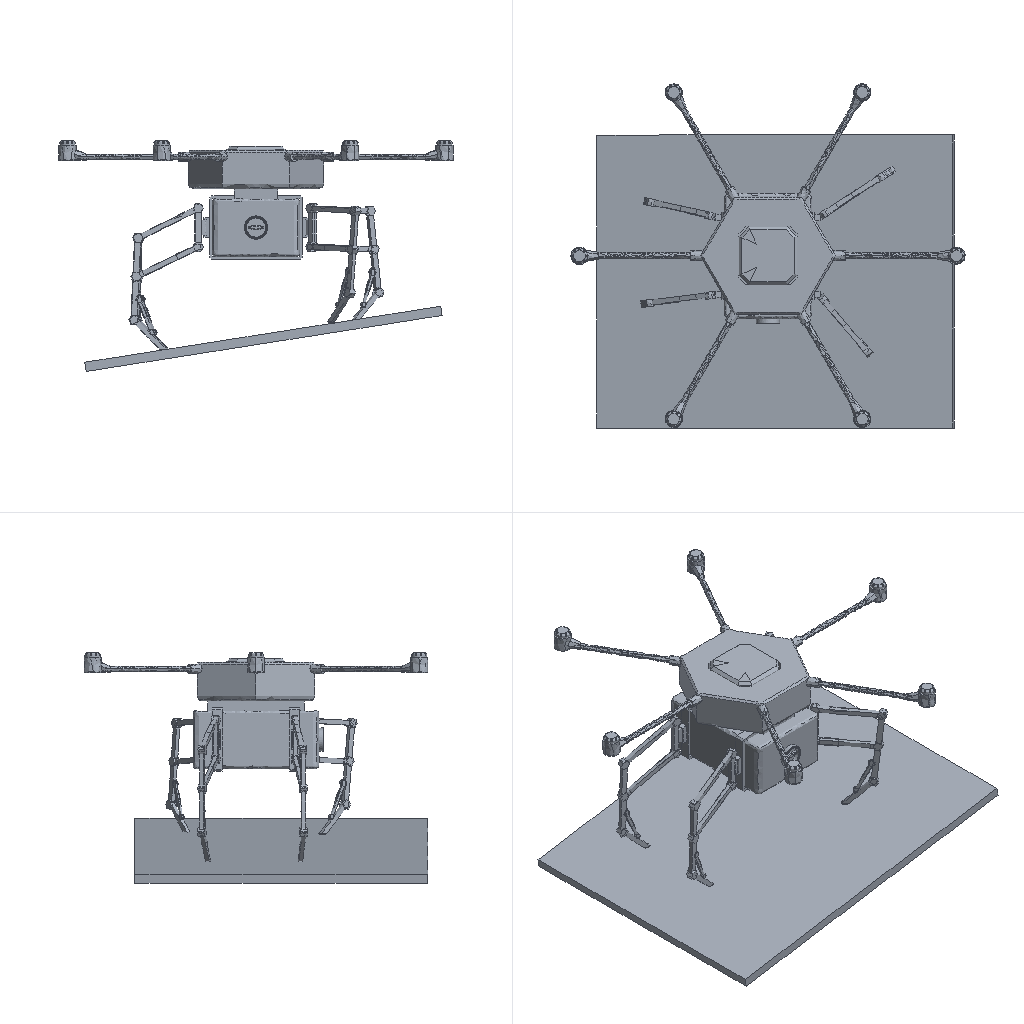Simulation study | ansys workbench
Ansys APDL input file, long lists of numbers shortened:
/batch
/config,noeldb,1     ! force off writing results to database
*get,_wallstrt,active,,time,wall
! ANSYS input file written by Workbench version 2022 R1
! File used for geometry attach:
/title,wbnew--____ (B5)
! ****** Begin Custom Load Command Snippet ******
/COM, ACT Extensions:
/COM,     LSDYNA, 2021.1
/COM,
! ****** End   Custom Load Command Snippet ******
*DIM,_wb_ProjectScratch_dir,string,248
_wb_ProjectScratch_dir(1) = ''
*DIM,_wb_SolverFiles_dir,string,248
_wb_SolverFiles_dir(1) = ''
*DIM,_wb_userfiles_dir,string,248
_wb_userfiles_dir(1) = ''
/com,--- Data in consistent NMM units. See Solving Units in the help system for more information.
/units,MPA
/nopr
/wb,file,start              !  signify a WB generated input file
/prep7
! Turn off shape checking because checks already performed inside WB mesher.
! See help system for more information.
SHPP,OFF,,NOWARN
/nolist
etcon,set             ! allow ANSYS to choose best KEYOP's for 180x elements, resets any applicable keyopt to MAPDL defaults
/com,*********** Nodes for the whole assembly ***********
nblock,3,,112162
(1i9,3e20.9e3)
        1    -4.940198886E+03     5.343852573E+02    -1.661004366E+03
! (101965 more lines like these left out)
-1
/wb,elem,start            !  set before creation of elements
/com,*********** Elements for Body 1 "xuanyi|dianjizhijia|Chamfer.1" ***********
et,1,187
eblock,19,solid,,480
(19i9)
        1        1        1        1        0        0        0        0       10        0    20386    35761    35765    35869    35796    35956    35983    35959    35957
! (959 more lines like these left out)
-1
/com,*********** Elements for Body 2 "xuanyi|jibi|Pad.1" ***********
et,2,187
eblock,19,solid,,1308
(19i9)
        2        2        2        2        0        0        0        0       10        0    42182    78115    78116    78183    78275    79189    79200    79191    79195
! (2615 more lines like these left out)
-1
/com,*********** Elements for Body 3 "xuanyi|xuanyidianji|CircPattern.1" ***********
et,3,187
eblock,19,solid,,3493
(19i9)
        3        3        3        3        0        0        0        0       10        0     9130    17713    17730    17812    17778    22405    22473    22409    22406
! (6985 more lines like these left out)
-1
/com,*********** Elements for Body 4 "xuanyi|dianjizhijia|Chamfer.1[2]" ***********
et,4,187
eblock,19,solid,,480
(19i9)
        4        4        4        4        0        0        0        0       10        0     4107     6963     6967     7071     6998     7158     7185     7161     7159
! (959 more lines like these left out)
-1
/com,*********** Elements for Body 5 "xuanyi|jibi|Pad.1[2]" ***********
et,5,187
eblock,19,solid,,1308
(19i9)
        5        5        5        5        0        0        0        0       10        0    40874    75480    75481    75548    75640    76554    76565    76556    76560
! (2615 more lines like these left out)
-1
! (50 more sections like these left out)
/wb,elem,end               !  done creating elements
/com,*********** Send User Defined Coordinate System(s) ***********
csys,0
toffst,273.15,  ! Temperature offset from absolute zero
/com,*********** Set Reference Temperature ***********
tref,22.
/wb,mat,start              !  starting to send materials
/com,*********** Send Materials ***********
Temperature = 'TEMP' ! Temperature
MP,DENS,1,7.85e-09,	! tonne mm^-3
MP,ALPX,1,1.2e-05,	! C^-1
MP,C,1,434000000,	! mm^2 s^-2 C^-1
MP,KXX,1,60.5,	! tonne mm s^-3 C^-1
MP,RSVX,1,0.00017,	! ohm mm
MP,EX,1,200000,	! tonne s^-2 mm^-1
MP,NUXY,1,0.3,
MP,MURX,1,10000,
Temperature = 'TEMP' ! Temperature
MP,DENS,2,7.85e-09,	! tonne mm^-3
MP,ALPX,2,1.2e-05,	! C^-1
MP,C,2,434000000,	! mm^2 s^-2 C^-1
MP,KXX,2,60.5,	! tonne mm s^-3 C^-1
MP,RSVX,2,0.00017,	! ohm mm
MP,EX,2,200000,	! tonne s^-2 mm^-1
MP,NUXY,2,0.3,
MP,MURX,2,10000,
Temperature = 'TEMP' ! Temperature
MP,DENS,3,7.85e-09,	! tonne mm^-3
MP,ALPX,3,1.2e-05,	! C^-1
MP,C,3,434000000,	! mm^2 s^-2 C^-1
MP,KXX,3,60.5,	! tonne mm s^-3 C^-1
MP,RSVX,3,0.00017,	! ohm mm
MP,EX,3,200000,	! tonne s^-2 mm^-1
MP,NUXY,3,0.3,
MP,MURX,3,10000,
Temperature = 'TEMP' ! Temperature
MP,DENS,4,7.85e-09,	! tonne mm^-3
MP,ALPX,4,1.2e-05,	! C^-1
MP,C,4,434000000,	! mm^2 s^-2 C^-1
MP,KXX,4,60.5,	! tonne mm s^-3 C^-1
MP,RSVX,4,0.00017,	! ohm mm
MP,EX,4,200000,	! tonne s^-2 mm^-1
MP,NUXY,4,0.3,
MP,MURX,4,10000,
Temperature = 'TEMP' ! Temperature
MP,DENS,5,7.85e-09,	! tonne mm^-3
MP,ALPX,5,1.2e-05,	! C^-1
MP,C,5,434000000,	! mm^2 s^-2 C^-1
MP,KXX,5,60.5,	! tonne mm s^-3 C^-1
MP,RSVX,5,0.00017,	! ohm mm
MP,EX,5,200000,	! tonne s^-2 mm^-1
MP,NUXY,5,0.3,
MP,MURX,5,10000,
Temperature = 'TEMP' ! Temperature
MP,DENS,6,7.85e-09,	! tonne mm^-3
MP,ALPX,6,1.2e-05,	! C^-1
MP,C,6,434000000,	! mm^2 s^-2 C^-1
MP,KXX,6,60.5,	! tonne mm s^-3 C^-1
MP,RSVX,6,0.00017,	! ohm mm
MP,EX,6,200000,	! tonne s^-2 mm^-1
MP,NUXY,6,0.3,
MP,MURX,6,10000,
Temperature = 'TEMP' ! Temperature
MP,DENS,7,7.85e-09,	! tonne mm^-3
MP,ALPX,7,1.2e-05,	! C^-1
MP,C,7,434000000,	! mm^2 s^-2 C^-1
MP,KXX,7,60.5,	! tonne mm s^-3 C^-1
MP,RSVX,7,0.00017,	! ohm mm
MP,EX,7,200000,	! tonne s^-2 mm^-1
MP,NUXY,7,0.3,
MP,MURX,7,10000,
Temperature = 'TEMP' ! Temperature
MP,DENS,8,7.85e-09,	! tonne mm^-3
MP,ALPX,8,1.2e-05,	! C^-1
MP,C,8,434000000,	! mm^2 s^-2 C^-1
MP,KXX,8,60.5,	! tonne mm s^-3 C^-1
MP,RSVX,8,0.00017,	! ohm mm
MP,EX,8,200000,	! tonne s^-2 mm^-1
MP,NUXY,8,0.3,
MP,MURX,8,10000,
Temperature = 'TEMP' ! Temperature
MP,DENS,9,7.85e-09,	! tonne mm^-3
MP,ALPX,9,1.2e-05,	! C^-1
MP,C,9,434000000,	! mm^2 s^-2 C^-1
MP,KXX,9,60.5,	! tonne mm s^-3 C^-1
MP,RSVX,9,0.00017,	! ohm mm
MP,EX,9,200000,	! tonne s^-2 mm^-1
! (416 more lines like these left out)
/wb,mat,end                !  done sending materials
!************************* Model Summary ********************
!xuanyi|dianjizhijia|Chamfer.1,	结构钢,	matid,	1
!xuanyi|jibi|Pad.1,	结构钢,	matid,	2
!xuanyi|xuanyidianji|CircPattern.1,	结构钢,	matid,	3
! (54 more lines like these left out)
*get,_xmin,node,,mnloc,x
*get,_ymin,node,,mnloc,y
*get,_zmin,node,,mnloc,z
*get,_xmax,node,,mxloc,x
*get,_ymax,node,,mxloc,y
*get,_zmax,node,,mxloc,z
_ASMDIAG=(_xmax-_xmin)*(_xmax-_xmin)+(_ymax-_ymin)*(_ymax-_ymin)+(_zmax-_zmin)*(_zmax-_zmin)
_ASMDIAG=SQRT(_ASMDIAG)
/wb,contact,start          !  starting to send contact
/com,*********** Create Contact "接触区域" ***********
/com,            Real Constant Set For Above Contact Is 57 & 56
*set,tid,57
*set,cid,56
r,tid
r,cid
et,tid,170
et,cid,174
eblock,10,,,60
(15i9)
    80841       57       57       57        0    35809    35902    35811    35811    36320    36340    35811    36314
! (59 more lines like these left out)
-1
eblock,10,,,60
(15i9)
    80901       56       56       56        0    35809    35902    35811    35811    36320    36340    35811    36314
! (59 more lines like these left out)
-1
eblock,10,,,74
(15i9)
    80961       56       57       56        0    78045    78052    78047    78047    78535    78544    78047    78533
! (73 more lines like these left out)
-1
eblock,10,,,74
(15i9)
    81035       57       56       57        0    78045    78052    78047    78047    78535    78544    78047    78533
! (73 more lines like these left out)
-1
keyo,cid,8,2               ! auto create asymmetric contact (from Program Controlled setting)
keyo,cid,10,0              ! adjust contact stiffness each NR iteration (from Program Controlled setting)
keyo,cid,12,5              ! bonded always
keyo,cid,18,1              ! small sliding turned on by application
keyo,cid,2,0               ! augmented Lagrange (from Program Controlled setting)
keyo,cid,4,0               ! on Gauss point (from Program Controlled setting)
keyo,cid,9,1               ! ignore initial gaps/penetration
keyo,cid,7,0               ! No Prediction
rmod,tid,3,10.      ! FKN
rmod,tid,5,0.       ! ICONT
rmod,tid,6,0.       ! PINB
rmod,tid,10,0.      ! CNOF
rmod,tid,12,0.      ! FKT
rmod,tid,36,230     ! WB DSID
rmod,cid,3,10.      ! FKN
rmod,cid,5,0.       ! ICONT
rmod,cid,6,0.       ! PINB
rmod,cid,10,0.      ! CNOF
rmod,cid,12,0.      ! FKT
rmod,cid,36,230     ! WB DSID
/com,*********** Create Contact "接触区域 2" ***********
/com,            Real Constant Set For Above Contact Is 59 & 58
*set,tid,59
*set,cid,58
r,tid
r,cid
et,tid,170
et,cid,174
eblock,10,,,78
(15i9)
    81109       59       59       59        0    35791    35793    35903    35903    36178    36198    35903    36183
! (77 more lines like these left out)
-1
eblock,10,,,78
(15i9)
    81187       58       58       58        0    35791    35793    35903    35903    36178    36198    35903    36183
! (77 more lines like these left out)
-1
eblock,10,,,254
(15i9)
    81265       58       59       58        0    17194    17404    17201    17201    19412    19464    17201    19408
! (253 more lines like these left out)
-1
eblock,10,,,254
(15i9)
    81519       59       58       59        0    17194    17404    17201    17201    19412    19464    17201    19408
! (253 more lines like these left out)
-1
keyo,cid,8,2               ! auto create asymmetric contact (from Program Controlled setting)
keyo,cid,10,0              ! adjust contact stiffness each NR iteration (from Program Controlled setting)
keyo,cid,12,5              ! bonded always
keyo,cid,18,1              ! small sliding turned on by application
keyo,cid,2,0               ! augmented Lagrange (from Program Controlled setting)
keyo,cid,4,0               ! on Gauss point (from Program Controlled setting)
keyo,cid,9,1               ! ignore initial gaps/penetration
keyo,cid,7,0               ! No Prediction
rmod,tid,3,10.      ! FKN
rmod,tid,5,0.       ! ICONT
rmod,tid,6,0.       ! PINB
rmod,tid,10,0.      ! CNOF
rmod,tid,12,0.      ! FKT
rmod,tid,36,233     ! WB DSID
rmod,cid,3,10.      ! FKN
rmod,cid,5,0.       ! ICONT
rmod,cid,6,0.       ! PINB
rmod,cid,10,0.      ! CNOF
rmod,cid,12,0.      ! FKT
rmod,cid,36,233     ! WB DSID
/com,*********** Create Contact "接触区域 3" ***********
/com,            Real Constant Set For Above Contact Is 61 & 60
*set,tid,61
*set,cid,60
r,tid
r,cid
et,tid,170
et,cid,174
eblock,10,,,85
(15i9)
    81773       61       61       61        0    78037    78044    78042    78042    78490    78519    78042    78489
! (84 more lines like these left out)
-1
eblock,10,,,85
(15i9)
    81858       60       60       60        0    78037    78044    78042    78042    78490    78519    78042    78489
! (84 more lines like these left out)
-1
eblock,10,,,60
(15i9)
    81943       60       61       60        0    48527    49307    48530    48530    53320    53345    48530    53318
! (59 more lines like these left out)
-1
eblock,10,,,60
(15i9)
    82003       61       60       61        0    48527    49307    48530    48530    53320    53345    48530    53318
! (59 more lines like these left out)
-1
keyo,cid,8,2               ! auto create asymmetric contact (from Program Controlled setting)
keyo,cid,10,0              ! adjust contact stiffness each NR iteration (from Program Controlled setting)
keyo,cid,12,5              ! bonded always
keyo,cid,18,1              ! small sliding turned on by application
keyo,cid,2,0               ! augmented Lagrange (from Program Controlled setting)
keyo,cid,4,0               ! on Gauss point (from Program Controlled setting)
keyo,cid,9,1               ! ignore initial gaps/penetration
keyo,cid,7,0               ! No Prediction
rmod,tid,3,10.      ! FKN
rmod,tid,5,0.       ! ICONT
rmod,tid,6,0.       ! PINB
rmod,tid,10,0.      ! CNOF
rmod,tid,12,0.      ! FKT
rmod,tid,36,236     ! WB DSID
rmod,cid,3,10.      ! FKN
rmod,cid,5,0.       ! ICONT
rmod,cid,6,0.       ! PINB
rmod,cid,10,0.      ! CNOF
rmod,cid,12,0.      ! FKT
rmod,cid,36,236     ! WB DSID
/com,*********** Create Contact "接触区域 8" ***********
/com,            Real Constant Set For Above Contact Is 63 & 62
*set,tid,63
*set,cid,62
r,tid
r,cid
et,tid,170
et,cid,174
eblock,10,,,60
(15i9)
    82063       63       63       63        0     7011     7104     7013     7013     7522     7542     7013     7516
! (59 more lines like these left out)
-1
eblock,10,,,60
(15i9)
    82123       62       62       62        0     7011     7104     7013     7013     7522     7542     7013     7516
! (59 more lines like these left out)
-1
eblock,10,,,74
(15i9)
    82183       62       63       62        0    75410    75417    75412    75412    75900    75909    75412    75898
! (73 more lines like these left out)
-1
eblock,10,,,74
(15i9)
    82257       63       62       63        0    75410    75417    75412    75412    75900    75909    75412    75898
! (73 more lines like these left out)
-1
keyo,cid,8,2               ! auto create asymmetric contact (from Program Controlled setting)
keyo,cid,10,0              ! adjust contact stiffness each NR iteration (from Program Controlled setting)
keyo,cid,12,5              ! bonded always
keyo,cid,18,1              ! small sliding turned on by application
keyo,cid,2,0               ! augmented Lagrange (from Program Controlled setting)
keyo,cid,4,0               ! on Gauss point (from Program Controlled setting)
keyo,cid,9,1               ! ignore initial gaps/penetration
keyo,cid,7,0               ! No Prediction
rmod,tid,3,10.      ! FKN
rmod,tid,5,0.       ! ICONT
rmod,tid,6,0.       ! PINB
rmod,tid,10,0.      ! CNOF
rmod,tid,12,0.      ! FKT
rmod,tid,36,251     ! WB DSID
rmod,cid,3,10.      ! FKN
rmod,cid,5,0.       ! ICONT
rmod,cid,6,0.       ! PINB
rmod,cid,10,0.      ! CNOF
rmod,cid,12,0.      ! FKT
rmod,cid,36,251     ! WB DSID
/com,*********** Create Contact "接触区域 9" ***********
/com,            Real Constant Set For Above Contact Is 65 & 64
*set,tid,65
*set,cid,64
r,tid
r,cid
et,tid,170
et,cid,174
eblock,10,,,78
(15i9)
    82331       65       65       65        0     6993     6995     7105     7105     7380     7400     7105     7385
! (77 more lines like these left out)
-1
eblock,10,,,78
(15i9)
    82409       64       64       64        0     6993     6995     7105     7105     7380     7400     7105     7385
! (77 more lines like these left out)
-1
eblock,10,,,254
(15i9)
    82487       64       65       64        0      546      756      553      553     2764     2816      553     2760
! (253 more lines like these left out)
-1
eblock,10,,,254
(15i9)
    82741       65       64       65        0      546      756      553      553     2764     2816      553     2760
! (253 more lines like these left out)
-1
keyo,cid,8,2               ! auto create asymmetric contact (from Program Controlled setting)
keyo,cid,10,0              ! adjust contact stiffness each NR iteration (from Program Controlled setting)
keyo,cid,12,5              ! bonded always
keyo,cid,18,1              ! small sliding turned on by application
keyo,cid,2,0               ! augmented Lagrange (from Program Controlled setting)
keyo,cid,4,0               ! on Gauss point (from Program Controlled setting)
keyo,cid,9,1               ! ignore initial gaps/penetration
keyo,cid,7,0               ! No Prediction
rmod,tid,3,10.      ! FKN
rmod,tid,5,0.       ! ICONT
rmod,tid,6,0.       ! PINB
rmod,tid,10,0.      ! CNOF
rmod,tid,12,0.      ! FKT
rmod,tid,36,254     ! WB DSID
rmod,cid,3,10.      ! FKN
rmod,cid,5,0.       ! ICONT
rmod,cid,6,0.       ! PINB
rmod,cid,10,0.      ! CNOF
rmod,cid,12,0.      ! FKT
rmod,cid,36,254     ! WB DSID
! (58 more sections like these left out)
/wb,contact,end            !  done creating contacts
/golist
/wb,load,start             !  starting to send loads
/com,*********** Fixed Supports ***********
CMBLOCK,_FIXEDSU,NODE,     7883
(8i10)
         7        14        17        22        23        24        28        29
! (985 more lines like these left out)
cmsel,s,_FIXEDSU
d,all,all
nsel,all
/com,*********** Define Force Using Surface Effect Elements ***********
local,12,0,0.,0.,0.,0.,0.,0.
csys,0
et,182,154
eblock,10,,,224
(15i9)
    93535      182      182      182       12    10610    10562    10561    10561    10825    10814    10561    10816
! (223 more lines like these left out)
-1
esel,s,type,,182
keyop,182,2,1                ! Apply load in local coordinate system
keyop,182,7,1                ! Use original area so load is constant in large deformation
esel,all
/gst,on,on
fini
*get,_numnode,node,0,count
*get,_numelem,elem,0,count
*get, _MAXELEMNUM, elem, 0, NUM, MAX
*get, _MAXNODENUM, node, 0, NUM, MAX
*get, _MAXELEMTYPE, etyp, 0, NUM, MAX
*get, _MAXREALCONST, real, 0, NUM, MAX
/go
/wb,load,end               !  done creating loads
/com,--- Number of total nodes = %_numnode%
/com,--- Number of contact elements = 12918
/com,--- Number of spring elements = 0
/com,--- Number of bearing elements = 0
/com,--- Number of solid elements = 55344
/com,--- Number of condensed parts = 0
/com,--- Number of total elements = %_numelem%
*get,_wallbsol,active,,time,wall
/com,****************************************************************************
/com,*************************    SOLUTION       ********************************
/com,****************************************************************************
/solu
antype,0                   ! static analysis
_thickRatio=0.164   ! Ratio of thick parts in the model
eqsl,sparse,,,,,1
cntr,print,1               ! print out contact info and also make no initial contact an error
dmpoption,emat,no             ! Don't combine emat file for DANSYS
dmpoption,esav,no             ! Don't combine esav file for DANSYS
nldiag,cont,iter           ! print out contact info each equilibrium iteration
rescontrol,,none                 ! Do not keep any restart files
/com,****************************************************
/com,******************* SOLVE FOR LS 1 OF 1 ****************
esel,s,type,,182
nsle
sfe,all,1,pres,1,0.
sfe,all,2,pres,1,-8.39440322781677e-009
sfe,all,3,pres,1,-14.087
nsel,all
esel,all
/nopr
/gopr
nsub,1,1,1
time,1.
outres,erase
outres,all,none
outres,nsol,all,
outres,rsol,all
outres,eangl,all
outres,etmp,all
outres,veng,all
outres,strs,all,
outres,epel,all,
outres,eppl,all,
outres,cont,all,
! *********** WB SOLVE COMMAND ***********
! check interactive state
*get,ANSINTER_,active,,int
*if,ANSINTER_,ne,0,then
/eof
*endif
solve
/com *************** Write FE CONNECTORS *********
CEWRITE,file,ce,,INTE
/com,****************************************************
/com,*************** FINISHED SOLVE FOR LS 1 *************
*get,_wallasol,active,,time,wall
/nopr
*get,_numnode,node,0,count
*get,_numelem,elem,0,count
*get, _MAXELEMNUM, elem, 0, NUM, MAX
*get, _MAXNODENUM, node, 0, NUM, MAX,,,INTERNAL
*get, _MAXELEMTYPE, etyp, 0, NUM, MAX
*get, _MAXREALCONST, real, 0, NUM, MAX
/gopr
/post1
xmlo,ENCODING,ISO-8859-1
xmlo,parm
/xml,parm,xml
fini
/gopr
*get,_walldone,active,,time,wall
_preptime=(_wallbsol-_wallstrt)*3600
_solvtime=(_wallasol-_wallbsol)*3600
_posttime=(_walldone-_wallasol)*3600
_totaltim=(_walldone-_wallstrt)*3600
*get,_dlbratio,active,0,solu,dlbr
*get,_combtime,active,0,solu,comb
*get,_ssmode,active,0,solu,ssmm
*get,_ndofs,active,0,solu,ndof
*get,_sol_end_time,active,0,set,time
*if,_sol_end_time,eq,1.,then
/fclean				!clean distributed files
*endif
/com,--- Total number of nodes = %_numnode%
/com,--- Total number of elements = %_numelem%
/com,--- Element load balance ratio = %_dlbratio%
/com,--- Time to combine distributed files = %_combtime%
/com,--- Sparse memory mode = %_ssmode%
/com,--- Number of DOF = %_ndofs%
/wb,file,end               ! done with WB generated input